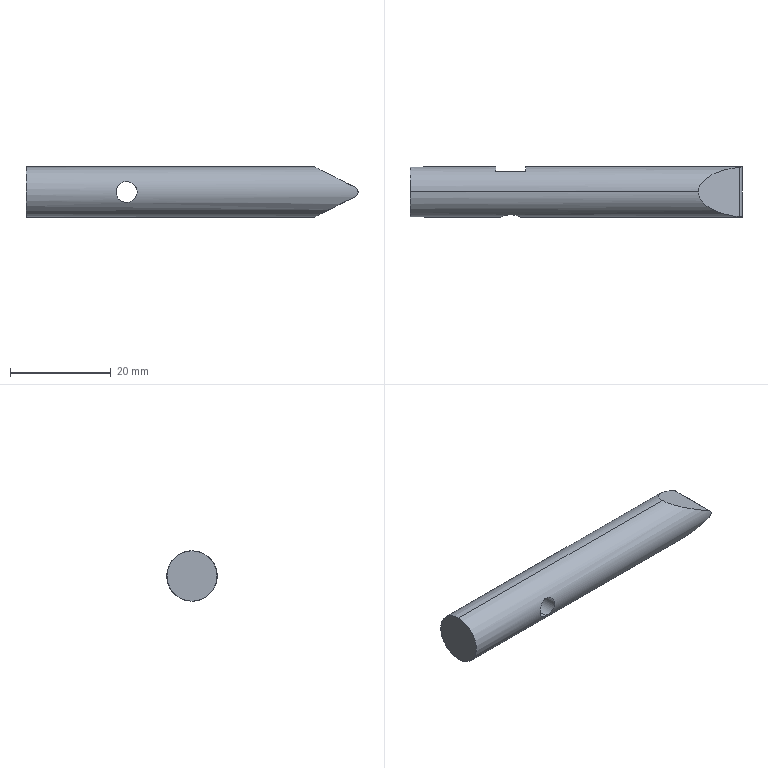Part | STEP file | BU-C04 | 1 solid | 11 faces | box 66 x 10 x 10 mm | volume 4793 mm3 | plane 6 | cylinder 5 | commonest cylinder face diameters 4.2 x2 10 x2 2 x1